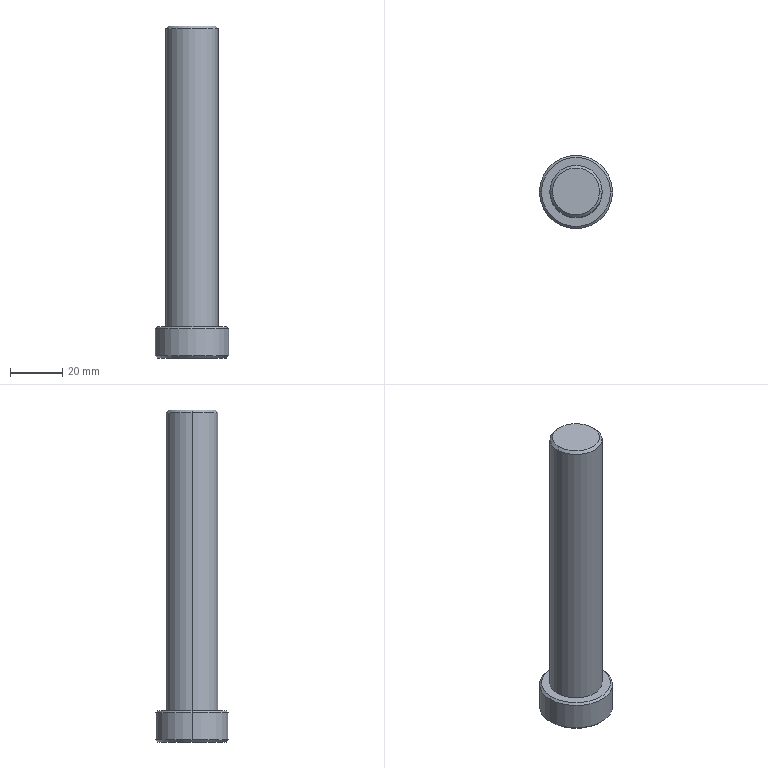Part | SolidWorks | features BaseBody 1 | 1 solid | 17 faces | box 28 x 28 x 127 mm | volume 42690 mm3 | cone 8 | cylinder 6 | plane 3 | commonest cylinder face diameters 6.8 x2 20 x2 28 x2
STEP:
#1=CARTESIAN_POINT('',(3.4,0.,19.75));
#2=VERTEX_POINT('',#1);
#3=CARTESIAN_POINT('',(-3.4,0.,19.75));
#4=VERTEX_POINT('',#3);
#5=CARTESIAN_POINT('',(0.,0.,19.75));
#6=DIRECTION('',(0.,0.,-1.));
#7=DIRECTION('',(-1.,0.,0.));
#8=AXIS2_PLACEMENT_3D('',#5,#6,#7);
#9=CIRCLE('',#8,3.4);
#10=EDGE_CURVE('',#2,#4,#9,.T.);
#11=ORIENTED_EDGE('',*,*,#10,.F.);
#12=CARTESIAN_POINT('',(3.4,0.,0.));
#13=VERTEX_POINT('',#12);
#14=CARTESIAN_POINT('',(3.4,0.,0.));
#15=DIRECTION('',(0.,0.,-1.));
#16=VECTOR('',#15,1000.);
#17=LINE('',#14,#16);
#18=EDGE_CURVE('',#2,#13,#17,.T.);
#19=ORIENTED_EDGE('',*,*,#18,.T.);
#20=CARTESIAN_POINT('',(-3.4,0.,0.));
#21=VERTEX_POINT('',#20);
#22=CARTESIAN_POINT('',(0.,0.,0.));
#23=DIRECTION('',(0.,0.,-1.));
#24=DIRECTION('',(-1.,0.,0.));
#25=AXIS2_PLACEMENT_3D('',#22,#23,#24);
#26=CIRCLE('',#25,3.4);
#27=EDGE_CURVE('',#13,#21,#26,.T.);
#28=ORIENTED_EDGE('',*,*,#27,.T.);
#29=CARTESIAN_POINT('',(-3.4,0.,0.));
#30=DIRECTION('',(0.,0.,-1.));
#31=VECTOR('',#30,1000.);
#32=LINE('',#29,#31);
#33=EDGE_CURVE('',#4,#21,#32,.T.);
#34=ORIENTED_EDGE('',*,*,#33,.F.);
#35=EDGE_LOOP('',(#11,#19,#28,#34));
#36=FACE_OUTER_BOUND('',#35,.T.);
#37=CARTESIAN_POINT('',(0.,0.,0.));
#38=DIRECTION('',(0.,0.,-1.));
#39=DIRECTION('',(-1.,0.,0.));
#40=AXIS2_PLACEMENT_3D('',#37,#38,#39);
#41=CYLINDRICAL_SURFACE('',#40,3.4);
#42=ADVANCED_FACE('',(#36),#41,.F.);
#43=CARTESIAN_POINT('',(0.,0.,21.793));
#44=VERTEX_POINT('',#43);
#45=CARTESIAN_POINT('',(-3.4,0.,19.75));
#46=DIRECTION('',(-0.8572,0.,-0.515));
#47=VECTOR('',#46,1000.);
#48=LINE('',#45,#47);
#49=EDGE_CURVE('',#44,#4,#48,.T.);
#50=ORIENTED_EDGE('',*,*,#49,.F.);
#51=CARTESIAN_POINT('',(3.4,0.,19.75));
#52=DIRECTION('',(0.8572,0.,-0.515));
#53=VECTOR('',#52,1000.);
#54=LINE('',#51,#53);
#55=EDGE_CURVE('',#44,#2,#54,.T.);
#56=ORIENTED_EDGE('',*,*,#55,.T.);
#57=ORIENTED_EDGE('',*,*,#10,.T.);
#58=EDGE_LOOP('',(#50,#56,#57));
#59=FACE_OUTER_BOUND('',#58,.T.);
#60=CARTESIAN_POINT('',(0.,0.,19.75));
#61=DIRECTION('',(0.,0.,-1.));
#62=DIRECTION('',(-1.,0.,0.));
#63=AXIS2_PLACEMENT_3D('',#60,#61,#62);
#64=CONICAL_SURFACE('',#63,3.4,1.03);
#65=ADVANCED_FACE('',(#59),#64,.F.);
#66=CARTESIAN_POINT('',(9.,0.,127.));
#67=VERTEX_POINT('',#66);
#68=CARTESIAN_POINT('',(-9.,0.,127.));
#69=VERTEX_POINT('',#68);
#70=CARTESIAN_POINT('',(0.,0.,127.));
#71=DIRECTION('',(0.,0.,1.));
#72=DIRECTION('',(1.,0.,0.));
#73=AXIS2_PLACEMENT_3D('',#70,#71,#72);
#74=CIRCLE('',#73,9.);
#75=EDGE_CURVE('',#67,#69,#74,.T.);
#76=ORIENTED_EDGE('',*,*,#75,.F.);
#77=CARTESIAN_POINT('',(10.,0.,126.));
#78=VERTEX_POINT('',#77);
#79=CARTESIAN_POINT('',(9.,0.,127.));
#80=DIRECTION('',(0.7071,0.,-0.7071));
#81=VECTOR('',#80,1000.);
#82=LINE('',#79,#81);
#83=EDGE_CURVE('',#67,#78,#82,.T.);
#84=ORIENTED_EDGE('',*,*,#83,.T.);
#85=CARTESIAN_POINT('',(-10.,0.,126.));
#86=VERTEX_POINT('',#85);
#87=CARTESIAN_POINT('',(0.,0.,126.));
#88=DIRECTION('',(0.,0.,-1.));
#89=DIRECTION('',(1.,0.,0.));
#90=AXIS2_PLACEMENT_3D('',#87,#88,#89);
#91=CIRCLE('',#90,10.);
#92=EDGE_CURVE('',#86,#78,#91,.T.);
#93=ORIENTED_EDGE('',*,*,#92,.F.);
#94=CARTESIAN_POINT('',(-9.,0.,127.));
#95=DIRECTION('',(-0.7071,0.,-0.7071));
#96=VECTOR('',#95,1000.);
#97=LINE('',#94,#96);
#98=EDGE_CURVE('',#69,#86,#97,.T.);
#99=ORIENTED_EDGE('',*,*,#98,.F.);
#100=EDGE_LOOP('',(#76,#84,#93,#99));
#101=FACE_OUTER_BOUND('',#100,.T.);
#102=CARTESIAN_POINT('',(0.,0.,127.));
#103=DIRECTION('',(0.,0.,-1.));
#104=DIRECTION('',(-1.,0.,0.));
#105=AXIS2_PLACEMENT_3D('',#102,#103,#104);
#106=CONICAL_SURFACE('',#105,9.,0.7854);
#107=ADVANCED_FACE('',(#101),#106,.T.);
#108=CARTESIAN_POINT('',(13.2,0.,12.));
#109=VERTEX_POINT('',#108);
#110=CARTESIAN_POINT('',(-13.2,0.,12.));
#111=VERTEX_POINT('',#110);
#112=CARTESIAN_POINT('',(0.,0.,12.));
#113=DIRECTION('',(0.,0.,1.));
#114=DIRECTION('',(1.,0.,0.));
#115=AXIS2_PLACEMENT_3D('',#112,#113,#114);
#116=CIRCLE('',#115,13.2);
#117=EDGE_CURVE('',#109,#111,#116,.T.);
#118=ORIENTED_EDGE('',*,*,#117,.F.);
#119=CARTESIAN_POINT('',(14.,0.,11.2));
#120=VERTEX_POINT('',#119);
#121=CARTESIAN_POINT('',(13.2,0.,12.));
#122=DIRECTION('',(0.7071,0.,-0.7071));
#123=VECTOR('',#122,1000.);
#124=LINE('',#121,#123);
#125=EDGE_CURVE('',#109,#120,#124,.T.);
#126=ORIENTED_EDGE('',*,*,#125,.T.);
#127=CARTESIAN_POINT('',(-14.,0.,11.2));
#128=VERTEX_POINT('',#127);
#129=CARTESIAN_POINT('',(0.,0.,11.2));
#130=DIRECTION('',(0.,0.,-1.));
#131=DIRECTION('',(1.,0.,0.));
#132=AXIS2_PLACEMENT_3D('',#129,#130,#131);
#133=CIRCLE('',#132,14.);
#134=EDGE_CURVE('',#128,#120,#133,.T.);
#135=ORIENTED_EDGE('',*,*,#134,.F.);
#136=CARTESIAN_POINT('',(-13.2,0.,12.));
#137=DIRECTION('',(-0.7071,0.,-0.7071));
#138=VECTOR('',#137,1000.);
#139=LINE('',#136,#138);
#140=EDGE_CURVE('',#111,#128,#139,.T.);
#141=ORIENTED_EDGE('',*,*,#140,.F.);
#142=EDGE_LOOP('',(#118,#126,#135,#141));
#143=FACE_OUTER_BOUND('',#142,.T.);
#144=CARTESIAN_POINT('',(0.,0.,12.));
#145=DIRECTION('',(0.,0.,-1.));
#146=DIRECTION('',(-1.,0.,0.));
#147=AXIS2_PLACEMENT_3D('',#144,#145,#146);
#148=CONICAL_SURFACE('',#147,13.2,0.7854);
#149=ADVANCED_FACE('',(#143),#148,.T.);
#150=CARTESIAN_POINT('',(-13.2,0.,0.));
#151=VERTEX_POINT('',#150);
#152=CARTESIAN_POINT('',(13.2,0.,0.));
#153=VERTEX_POINT('',#152);
#154=CARTESIAN_POINT('',(0.,0.,0.));
#155=DIRECTION('',(0.,0.,-1.));
#156=DIRECTION('',(1.,0.,0.));
#157=AXIS2_PLACEMENT_3D('',#154,#155,#156);
#158=CIRCLE('',#157,13.2);
#159=EDGE_CURVE('',#151,#153,#158,.T.);
#160=ORIENTED_EDGE('',*,*,#159,.F.);
#161=CARTESIAN_POINT('',(-14.,0.,0.8));
#162=VERTEX_POINT('',#161);
#163=CARTESIAN_POINT('',(-14.,0.,0.8));
#164=DIRECTION('',(-0.7071,0.,0.7071));
#165=VECTOR('',#164,1000.);
#166=LINE('',#163,#165);
#167=EDGE_CURVE('',#151,#162,#166,.T.);
#168=ORIENTED_EDGE('',*,*,#167,.T.);
#169=CARTESIAN_POINT('',(14.,0.,0.8));
#170=VERTEX_POINT('',#169);
#171=CARTESIAN_POINT('',(0.,0.,0.8));
#172=DIRECTION('',(0.,0.,1.));
#173=DIRECTION('',(1.,0.,0.));
#174=AXIS2_PLACEMENT_3D('',#171,#172,#173);
#175=CIRCLE('',#174,14.);
#176=EDGE_CURVE('',#170,#162,#175,.T.);
#177=ORIENTED_EDGE('',*,*,#176,.F.);
#178=CARTESIAN_POINT('',(14.,0.,0.8));
#179=DIRECTION('',(0.7071,0.,0.7071));
#180=VECTOR('',#179,1000.);
#181=LINE('',#178,#180);
#182=EDGE_CURVE('',#153,#170,#181,.T.);
#183=ORIENTED_EDGE('',*,*,#182,.F.);
#184=EDGE_LOOP('',(#160,#168,#177,#183));
#185=FACE_OUTER_BOUND('',#184,.T.);
#186=CARTESIAN_POINT('',(0.,0.,0.8));
#187=DIRECTION('',(0.,0.,1.));
#188=DIRECTION('',(1.,0.,0.));
#189=AXIS2_PLACEMENT_3D('',#186,#187,#188);
#190=CONICAL_SURFACE('',#189,14.,0.7854);
#191=ADVANCED_FACE('',(#185),#190,.T.);
#192=ORIENTED_EDGE('',*,*,#92,.T.);
#193=CARTESIAN_POINT('',(10.,0.,12.));
#194=VERTEX_POINT('',#193);
#195=CARTESIAN_POINT('',(10.,0.,127.));
#196=DIRECTION('',(0.,0.,-1.));
#197=VECTOR('',#196,1000.);
#198=LINE('',#195,#197);
#199=EDGE_CURVE('',#78,#194,#198,.T.);
#200=ORIENTED_EDGE('',*,*,#199,.T.);
#201=CARTESIAN_POINT('',(-10.,0.,12.));
#202=VERTEX_POINT('',#201);
#203=CARTESIAN_POINT('',(0.,0.,12.));
#204=DIRECTION('',(0.,0.,1.));
#205=DIRECTION('',(1.,0.,0.));
#206=AXIS2_PLACEMENT_3D('',#203,#204,#205);
#207=CIRCLE('',#206,10.);
#208=EDGE_CURVE('',#194,#202,#207,.T.);
#209=ORIENTED_EDGE('',*,*,#208,.T.);
#210=CARTESIAN_POINT('',(-10.,0.,127.));
#211=DIRECTION('',(0.,0.,-1.));
#212=VECTOR('',#211,1000.);
#213=LINE('',#210,#212);
#214=EDGE_CURVE('',#86,#202,#213,.T.);
#215=ORIENTED_EDGE('',*,*,#214,.F.);
#216=EDGE_LOOP('',(#192,#200,#209,#215));
#217=FACE_OUTER_BOUND('',#216,.T.);
#218=CARTESIAN_POINT('',(0.,0.,127.));
#219=DIRECTION('',(0.,0.,-1.));
#220=DIRECTION('',(-1.,0.,0.));
#221=AXIS2_PLACEMENT_3D('',#218,#219,#220);
#222=CYLINDRICAL_SURFACE('',#221,10.);
#223=ADVANCED_FACE('',(#217),#222,.T.);
#224=ORIENTED_EDGE('',*,*,#134,.T.);
#225=CARTESIAN_POINT('',(14.,0.,12.));
#226=DIRECTION('',(0.,0.,-1.));
#227=VECTOR('',#226,1000.);
#228=LINE('',#225,#227);
#229=EDGE_CURVE('',#120,#170,#228,.T.);
#230=ORIENTED_EDGE('',*,*,#229,.T.);
#231=ORIENTED_EDGE('',*,*,#176,.T.);
#232=CARTESIAN_POINT('',(-14.,0.,12.));
#233=DIRECTION('',(0.,0.,-1.));
#234=VECTOR('',#233,1000.);
#235=LINE('',#232,#234);
#236=EDGE_CURVE('',#128,#162,#235,.T.);
#237=ORIENTED_EDGE('',*,*,#236,.F.);
#238=EDGE_LOOP('',(#224,#230,#231,#237));
#239=FACE_OUTER_BOUND('',#238,.T.);
#240=CARTESIAN_POINT('',(0.,0.,12.));
#241=DIRECTION('',(0.,0.,-1.));
#242=DIRECTION('',(-1.,0.,0.));
#243=AXIS2_PLACEMENT_3D('',#240,#241,#242);
#244=CYLINDRICAL_SURFACE('',#243,14.);
#245=ADVANCED_FACE('',(#239),#244,.T.);
#246=ORIENTED_EDGE('',*,*,#229,.F.);
#247=CARTESIAN_POINT('',(0.,0.,11.2));
#248=DIRECTION('',(0.,0.,-1.));
#249=DIRECTION('',(1.,0.,0.));
#250=AXIS2_PLACEMENT_3D('',#247,#248,#249);
#251=CIRCLE('',#250,14.);
#252=EDGE_CURVE('',#120,#128,#251,.T.);
#253=ORIENTED_EDGE('',*,*,#252,.T.);
#254=ORIENTED_EDGE('',*,*,#236,.T.);
#255=CARTESIAN_POINT('',(0.,0.,0.8));
#256=DIRECTION('',(0.,0.,1.));
#257=DIRECTION('',(1.,0.,0.));
#258=AXIS2_PLACEMENT_3D('',#255,#256,#257);
#259=CIRCLE('',#258,14.);
#260=EDGE_CURVE('',#162,#170,#259,.T.);
#261=ORIENTED_EDGE('',*,*,#260,.T.);
#262=EDGE_LOOP('',(#246,#253,#254,#261));
#263=FACE_OUTER_BOUND('',#262,.T.);
#264=CARTESIAN_POINT('',(0.,0.,12.));
#265=DIRECTION('',(0.,0.,-1.));
#266=DIRECTION('',(-1.,0.,0.));
#267=AXIS2_PLACEMENT_3D('',#264,#265,#266);
#268=CYLINDRICAL_SURFACE('',#267,14.);
#269=ADVANCED_FACE('',(#263),#268,.T.);
#270=CARTESIAN_POINT('',(0.,0.,12.));
#271=DIRECTION('',(0.,0.,1.));
#272=DIRECTION('',(1.,0.,0.));
#273=AXIS2_PLACEMENT_3D('',#270,#271,#272);
#274=CIRCLE('',#273,13.2);
#275=EDGE_CURVE('',#111,#109,#274,.T.);
#276=ORIENTED_EDGE('',*,*,#275,.T.);
#277=ORIENTED_EDGE('',*,*,#117,.T.);
#278=EDGE_LOOP('',(#276,#277));
#279=FACE_OUTER_BOUND('',#278,.T.);
#280=CARTESIAN_POINT('',(0.,0.,12.));
#281=DIRECTION('',(0.,0.,1.));
#282=DIRECTION('',(1.,0.,0.));
#283=AXIS2_PLACEMENT_3D('',#280,#281,#282);
#284=CIRCLE('',#283,10.);
#285=EDGE_CURVE('',#202,#194,#284,.T.);
#286=ORIENTED_EDGE('',*,*,#285,.F.);
#287=ORIENTED_EDGE('',*,*,#208,.F.);
#288=EDGE_LOOP('',(#286,#287));
#289=FACE_BOUND('',#288,.T.);
#290=CARTESIAN_POINT('',(0.,0.,12.));
#291=DIRECTION('',(0.,0.,1.));
#292=DIRECTION('',(1.,0.,0.));
#293=AXIS2_PLACEMENT_3D('',#290,#291,#292);
#294=PLANE('',#293);
#295=ADVANCED_FACE('',(#279,#289),#294,.T.);
#296=CARTESIAN_POINT('',(0.,0.,0.));
#297=DIRECTION('',(0.,0.,-1.));
#298=DIRECTION('',(-1.,0.,0.));
#299=AXIS2_PLACEMENT_3D('',#296,#297,#298);
#300=CIRCLE('',#299,3.4);
#301=EDGE_CURVE('',#21,#13,#300,.T.);
#302=ORIENTED_EDGE('',*,*,#301,.F.);
#303=ORIENTED_EDGE('',*,*,#27,.F.);
#304=EDGE_LOOP('',(#302,#303));
#305=FACE_BOUND('',#304,.T.);
#306=CARTESIAN_POINT('',(0.,0.,0.));
#307=DIRECTION('',(0.,0.,-1.));
#308=DIRECTION('',(1.,0.,0.));
#309=AXIS2_PLACEMENT_3D('',#306,#307,#308);
#310=CIRCLE('',#309,13.2);
#311=EDGE_CURVE('',#153,#151,#310,.T.);
#312=ORIENTED_EDGE('',*,*,#311,.T.);
#313=ORIENTED_EDGE('',*,*,#159,.T.);
#314=EDGE_LOOP('',(#312,#313));
#315=FACE_OUTER_BOUND('',#314,.T.);
#316=CARTESIAN_POINT('',(0.,0.,0.));
#317=DIRECTION('',(0.,0.,1.));
#318=DIRECTION('',(1.,0.,0.));
#319=AXIS2_PLACEMENT_3D('',#316,#317,#318);
#320=PLANE('',#319);
#321=ADVANCED_FACE('',(#305,#315),#320,.F.);
#322=ORIENTED_EDGE('',*,*,#199,.F.);
#323=CARTESIAN_POINT('',(0.,0.,126.));
#324=DIRECTION('',(0.,0.,-1.));
#325=DIRECTION('',(1.,0.,0.));
#326=AXIS2_PLACEMENT_3D('',#323,#324,#325);
#327=CIRCLE('',#326,10.);
#328=EDGE_CURVE('',#78,#86,#327,.T.);
#329=ORIENTED_EDGE('',*,*,#328,.T.);
#330=ORIENTED_EDGE('',*,*,#214,.T.);
#331=ORIENTED_EDGE('',*,*,#285,.T.);
#332=EDGE_LOOP('',(#322,#329,#330,#331));
#333=FACE_OUTER_BOUND('',#332,.T.);
#334=CARTESIAN_POINT('',(0.,0.,127.));
#335=DIRECTION('',(0.,0.,-1.));
#336=DIRECTION('',(-1.,0.,0.));
#337=AXIS2_PLACEMENT_3D('',#334,#335,#336);
#338=CYLINDRICAL_SURFACE('',#337,10.);
#339=ADVANCED_FACE('',(#333),#338,.T.);
#340=CARTESIAN_POINT('',(0.,0.,127.));
#341=DIRECTION('',(0.,0.,1.));
#342=DIRECTION('',(1.,0.,0.));
#343=AXIS2_PLACEMENT_3D('',#340,#341,#342);
#344=CIRCLE('',#343,9.);
#345=EDGE_CURVE('',#69,#67,#344,.T.);
#346=ORIENTED_EDGE('',*,*,#345,.T.);
#347=ORIENTED_EDGE('',*,*,#75,.T.);
#348=EDGE_LOOP('',(#346,#347));
#349=FACE_OUTER_BOUND('',#348,.T.);
#350=CARTESIAN_POINT('',(0.,0.,127.));
#351=DIRECTION('',(0.,0.,1.));
#352=DIRECTION('',(1.,0.,0.));
#353=AXIS2_PLACEMENT_3D('',#350,#351,#352);
#354=PLANE('',#353);
#355=ADVANCED_FACE('',(#349),#354,.T.);
#356=ORIENTED_EDGE('',*,*,#167,.F.);
#357=ORIENTED_EDGE('',*,*,#311,.F.);
#358=ORIENTED_EDGE('',*,*,#182,.T.);
#359=ORIENTED_EDGE('',*,*,#260,.F.);
#360=EDGE_LOOP('',(#356,#357,#358,#359));
#361=FACE_OUTER_BOUND('',#360,.T.);
#362=CARTESIAN_POINT('',(0.,0.,0.8));
#363=DIRECTION('',(0.,0.,1.));
#364=DIRECTION('',(1.,0.,0.));
#365=AXIS2_PLACEMENT_3D('',#362,#363,#364);
#366=CONICAL_SURFACE('',#365,14.,0.7854);
#367=ADVANCED_FACE('',(#361),#366,.T.);
#368=ORIENTED_EDGE('',*,*,#125,.F.);
#369=ORIENTED_EDGE('',*,*,#275,.F.);
#370=ORIENTED_EDGE('',*,*,#140,.T.);
#371=ORIENTED_EDGE('',*,*,#252,.F.);
#372=EDGE_LOOP('',(#368,#369,#370,#371));
#373=FACE_OUTER_BOUND('',#372,.T.);
#374=CARTESIAN_POINT('',(0.,0.,12.));
#375=DIRECTION('',(0.,0.,-1.));
#376=DIRECTION('',(-1.,0.,0.));
#377=AXIS2_PLACEMENT_3D('',#374,#375,#376);
#378=CONICAL_SURFACE('',#377,13.2,0.7854);
#379=ADVANCED_FACE('',(#373),#378,.T.);
#380=ORIENTED_EDGE('',*,*,#83,.F.);
#381=ORIENTED_EDGE('',*,*,#345,.F.);
#382=ORIENTED_EDGE('',*,*,#98,.T.);
#383=ORIENTED_EDGE('',*,*,#328,.F.);
#384=EDGE_LOOP('',(#380,#381,#382,#383));
#385=FACE_OUTER_BOUND('',#384,.T.);
#386=CARTESIAN_POINT('',(0.,0.,127.));
#387=DIRECTION('',(0.,0.,-1.));
#388=DIRECTION('',(-1.,0.,0.));
#389=AXIS2_PLACEMENT_3D('',#386,#387,#388);
#390=CONICAL_SURFACE('',#389,9.,0.7854);
#391=ADVANCED_FACE('',(#385),#390,.T.);
#392=ORIENTED_EDGE('',*,*,#55,.F.);
#393=ORIENTED_EDGE('',*,*,#49,.T.);
#394=CARTESIAN_POINT('',(0.,0.,19.75));
#395=DIRECTION('',(0.,0.,-1.));
#396=DIRECTION('',(-1.,0.,0.));
#397=AXIS2_PLACEMENT_3D('',#394,#395,#396);
#398=CIRCLE('',#397,3.4);
#399=EDGE_CURVE('',#4,#2,#398,.T.);
#400=ORIENTED_EDGE('',*,*,#399,.T.);
#401=EDGE_LOOP('',(#392,#393,#400));
#402=FACE_OUTER_BOUND('',#401,.T.);
#403=CARTESIAN_POINT('',(0.,0.,19.75));
#404=DIRECTION('',(0.,0.,-1.));
#405=DIRECTION('',(-1.,0.,0.));
#406=AXIS2_PLACEMENT_3D('',#403,#404,#405);
#407=CONICAL_SURFACE('',#406,3.4,1.03);
#408=ADVANCED_FACE('',(#402),#407,.F.);
#409=ORIENTED_EDGE('',*,*,#18,.F.);
#410=ORIENTED_EDGE('',*,*,#399,.F.);
#411=ORIENTED_EDGE('',*,*,#33,.T.);
#412=ORIENTED_EDGE('',*,*,#301,.T.);
#413=EDGE_LOOP('',(#409,#410,#411,#412));
#414=FACE_OUTER_BOUND('',#413,.T.);
#415=CARTESIAN_POINT('',(0.,0.,0.));
#416=DIRECTION('',(0.,0.,-1.));
#417=DIRECTION('',(-1.,0.,0.));
#418=AXIS2_PLACEMENT_3D('',#415,#416,#417);
#419=CYLINDRICAL_SURFACE('',#418,3.4);
#420=ADVANCED_FACE('',(#414),#419,.F.);
#421=CLOSED_SHELL('',(#42,#65,#107,#149,#191,#223,#245,#269,#295,#321,#339,#355,#367,#379,#391,#408,#420));
#422=MANIFOLD_SOLID_BREP('',#421);
#423=CARTESIAN_POINT('',(0.,0.,0.));
#424=DIRECTION('',(0.,0.,1.));
#425=DIRECTION('',(1.,0.,0.));
#426=AXIS2_PLACEMENT_3D('',#423,#424,#425);
#427=(LENGTH_UNIT()NAMED_UNIT(*)SI_UNIT(.MILLI.,.METRE.));
#428=UNCERTAINTY_MEASURE_WITH_UNIT(LENGTH_MEASURE(0.00001),#427,'','');
#429=(NAMED_UNIT(*)PLANE_ANGLE_UNIT()SI_UNIT($,.RADIAN.));
#430=(NAMED_UNIT(*)SI_UNIT($,.STERADIAN.)SOLID_ANGLE_UNIT());
#431=(GEOMETRIC_REPRESENTATION_CONTEXT(3)GLOBAL_UNCERTAINTY_ASSIGNED_CONTEXT((#428))GLOBAL_UNIT_ASSIGNED_CONTEXT((#427,#429,#430))REPRESENTATION_CONTEXT('',''));
#432=ADVANCED_BREP_SHAPE_REPRESENTATION('',(#422,#426),#431);